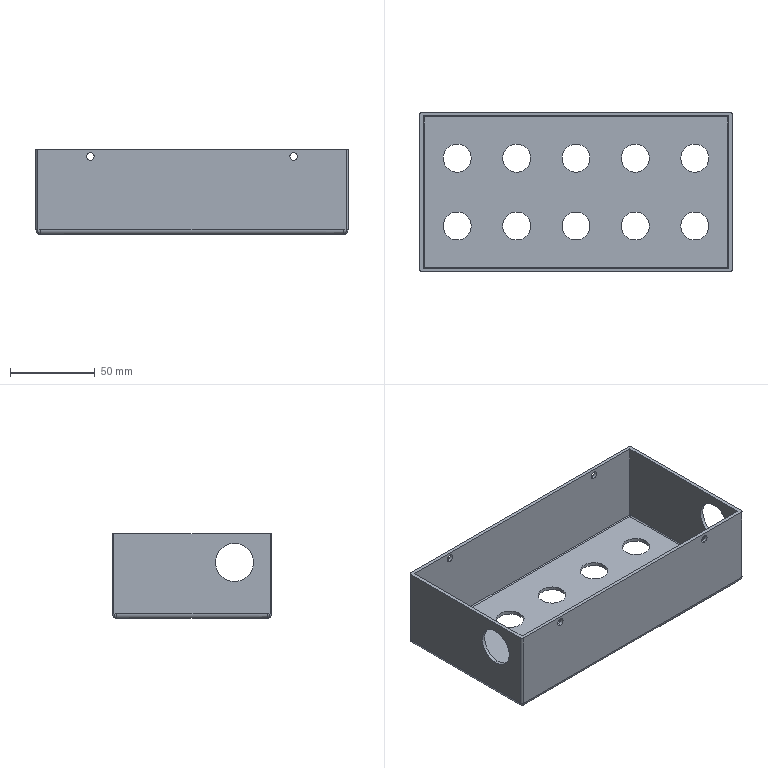Part | STEP file | Indicator light board | 1 solid | 75 faces | box 184 x 94 x 50 mm | volume 80341 mm3 | cylinder 44 | spline 20 | plane 11 | commonest cylinder face diameters 16.5 x20 4.5 x8 1.473 x4 2 x4 5.473 x4 22.5 x4